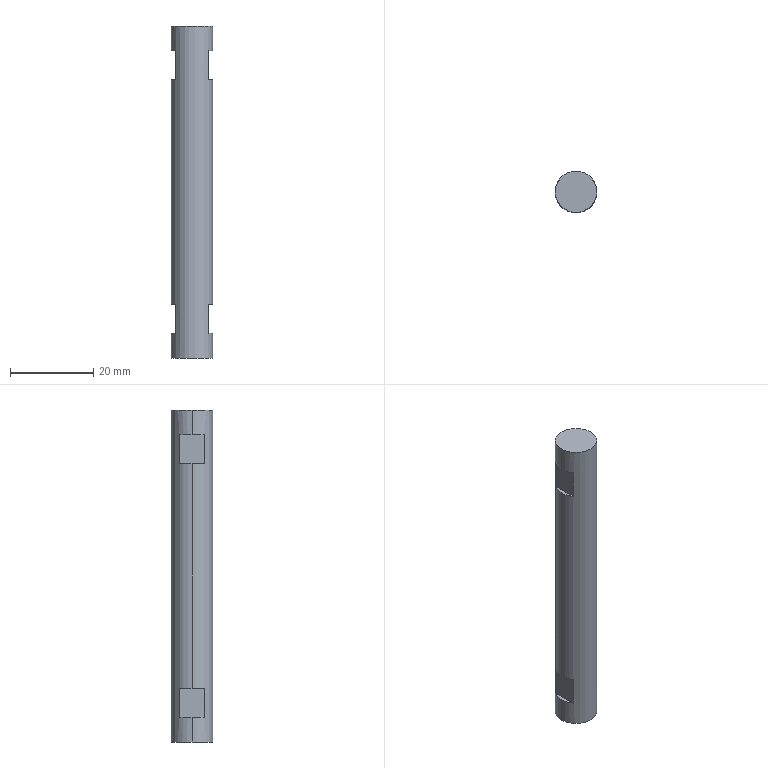Part | STEP file | GLSJ-10-19_default | 1 solid | 20 faces | box 10 x 10 x 80 mm | volume 5991 mm3 | plane 14 | cylinder 4 | cone 2 | commonest cylinder face diameters 4.2 x2 10 x2
STEP:
#1=CARTESIAN_POINT('',(0.,0.,0.));
#2=DIRECTION('',(0.,0.,1.));
#3=DIRECTION('',(1.,0.,0.));
#4=AXIS2_PLACEMENT_3D('',#1,#2,#3);
#5=CARTESIAN_POINT('',(-2.1,0.,12.4));
#6=VERTEX_POINT('',#5);
#7=CARTESIAN_POINT('',(-2.1,0.,0.));
#8=VERTEX_POINT('',#7);
#9=CARTESIAN_POINT('',(-2.1,0.,0.));
#10=DIRECTION('',(0.,0.,-1.));
#11=VECTOR('',#10,1.);
#12=LINE('',#9,#11);
#13=CARTESIAN_POINT('',(0.,0.,0.));
#14=DIRECTION('',(0.,0.,-1.));
#15=DIRECTION('',(-1.,0.,0.));
#16=AXIS2_PLACEMENT_3D('',#13,#14,#15);
#17=CYLINDRICAL_SURFACE('',#16,2.1);
#18=CARTESIAN_POINT('',(6.283,0.));
#19=DIRECTION('',(0.,1.));
#20=VECTOR('',#19,1.);
#21=LINE('',#18,#20);
#22=(GEOMETRIC_REPRESENTATION_CONTEXT(2)PARAMETRIC_REPRESENTATION_CONTEXT()REPRESENTATION_CONTEXT('',''));
#23=DEFINITIONAL_REPRESENTATION('',(#21),#22);
#24=PCURVE('',#17,#23);
#25=CARTESIAN_POINT('',(0.,0.,0.));
#26=DIRECTION('',(0.,0.,-1.));
#27=DIRECTION('',(-1.,0.,0.));
#28=AXIS2_PLACEMENT_3D('',#25,#26,#27);
#29=CYLINDRICAL_SURFACE('',#28,2.1);
#30=CARTESIAN_POINT('',(0.,0.));
#31=DIRECTION('',(0.,1.));
#32=VECTOR('',#31,1.);
#33=LINE('',#30,#32);
#34=(GEOMETRIC_REPRESENTATION_CONTEXT(2)PARAMETRIC_REPRESENTATION_CONTEXT()REPRESENTATION_CONTEXT('',''));
#35=DEFINITIONAL_REPRESENTATION('',(#33),#34);
#36=PCURVE('',#29,#35);
#37=SURFACE_CURVE('',#12,(#24,#36),.PCURVE_S1.);
#38=EDGE_CURVE('',#6,#8,#37,.T.);
#39=ORIENTED_EDGE('',*,*,#38,.T.);
#40=CARTESIAN_POINT('',(2.1,0.,0.));
#41=VERTEX_POINT('',#40);
#42=CARTESIAN_POINT('',(0.,0.,0.));
#43=DIRECTION('',(0.,0.,-1.));
#44=DIRECTION('',(-1.,0.,0.));
#45=AXIS2_PLACEMENT_3D('',#42,#43,#44);
#46=CIRCLE('',#45,2.1);
#47=CARTESIAN_POINT('',(0.,0.));
#48=DIRECTION('',(1.,0.));
#49=VECTOR('',#48,1.);
#50=LINE('',#47,#49);
#51=(GEOMETRIC_REPRESENTATION_CONTEXT(2)PARAMETRIC_REPRESENTATION_CONTEXT()REPRESENTATION_CONTEXT('',''));
#52=DEFINITIONAL_REPRESENTATION('',(#50),#51);
#53=PCURVE('',#17,#52);
#54=CARTESIAN_POINT('',(0.,0.,0.));
#55=DIRECTION('',(0.,0.,1.));
#56=DIRECTION('',(1.,0.,0.));
#57=AXIS2_PLACEMENT_3D('',#54,#55,#56);
#58=PLANE('',#57);
#59=CARTESIAN_POINT('',(-2.1,0.));
#60=CARTESIAN_POINT('',(-2.1,3.637));
#61=CARTESIAN_POINT('',(1.05,1.819));
#62=CARTESIAN_POINT('',(4.2,0.));
#63=CARTESIAN_POINT('',(1.05,-1.819));
#64=CARTESIAN_POINT('',(-2.1,-3.637));
#65=CARTESIAN_POINT('',(-2.1,0.));
#66=(BOUNDED_CURVE()B_SPLINE_CURVE(2,(#59,#60,#61,#62,#63,#64,#65),.UNSPECIFIED.,.T.,.F.)B_SPLINE_CURVE_WITH_KNOTS((1,2,2,2,2,1),(-2.094,0.,2.094,4.189,6.283,8.378),.UNSPECIFIED.)CURVE()GEOMETRIC_REPRESENTATION_ITEM()RATIONAL_B_SPLINE_CURVE((1.,0.5,1.,0.5,1.,0.5,1.))REPRESENTATION_ITEM(''));
#67=(GEOMETRIC_REPRESENTATION_CONTEXT(2)PARAMETRIC_REPRESENTATION_CONTEXT()REPRESENTATION_CONTEXT('',''));
#68=DEFINITIONAL_REPRESENTATION('',(#66),#67);
#69=PCURVE('',#58,#68);
#70=SURFACE_CURVE('',#46,(#53,#69),.PCURVE_S1.);
#71=EDGE_CURVE('',#41,#8,#70,.T.);
#72=ORIENTED_EDGE('',*,*,#71,.F.);
#73=CARTESIAN_POINT('',(2.1,0.,12.4));
#74=VERTEX_POINT('',#73);
#75=CARTESIAN_POINT('',(2.1,0.,0.));
#76=DIRECTION('',(0.,0.,-1.));
#77=VECTOR('',#76,1.);
#78=LINE('',#75,#77);
#79=CARTESIAN_POINT('',(3.142,0.));
#80=DIRECTION('',(0.,1.));
#81=VECTOR('',#80,1.);
#82=LINE('',#79,#81);
#83=(GEOMETRIC_REPRESENTATION_CONTEXT(2)PARAMETRIC_REPRESENTATION_CONTEXT()REPRESENTATION_CONTEXT('',''));
#84=DEFINITIONAL_REPRESENTATION('',(#82),#83);
#85=PCURVE('',#17,#84);
#86=CARTESIAN_POINT('',(3.142,0.));
#87=DIRECTION('',(0.,1.));
#88=VECTOR('',#87,1.);
#89=LINE('',#86,#88);
#90=(GEOMETRIC_REPRESENTATION_CONTEXT(2)PARAMETRIC_REPRESENTATION_CONTEXT()REPRESENTATION_CONTEXT('',''));
#91=DEFINITIONAL_REPRESENTATION('',(#89),#90);
#92=PCURVE('',#29,#91);
#93=SURFACE_CURVE('',#78,(#85,#92),.PCURVE_S1.);
#94=EDGE_CURVE('',#74,#41,#93,.T.);
#95=ORIENTED_EDGE('',*,*,#94,.F.);
#96=CARTESIAN_POINT('',(0.,0.,12.4));
#97=DIRECTION('',(0.,0.,-1.));
#98=DIRECTION('',(-1.,0.,0.));
#99=AXIS2_PLACEMENT_3D('',#96,#97,#98);
#100=CIRCLE('',#99,2.1);
#101=CARTESIAN_POINT('',(0.,-12.4));
#102=DIRECTION('',(1.,0.));
#103=VECTOR('',#102,1.);
#104=LINE('',#101,#103);
#105=(GEOMETRIC_REPRESENTATION_CONTEXT(2)PARAMETRIC_REPRESENTATION_CONTEXT()REPRESENTATION_CONTEXT('',''));
#106=DEFINITIONAL_REPRESENTATION('',(#104),#105);
#107=PCURVE('',#17,#106);
#108=CARTESIAN_POINT('',(0.,0.,12.4));
#109=DIRECTION('',(0.,0.,-1.));
#110=DIRECTION('',(-1.,0.,0.));
#111=AXIS2_PLACEMENT_3D('',#108,#109,#110);
#112=CONICAL_SURFACE('',#111,2.1,1.03);
#113=CARTESIAN_POINT('',(0.,0.));
#114=DIRECTION('',(1.,0.));
#115=VECTOR('',#114,1.);
#116=LINE('',#113,#115);
#117=(GEOMETRIC_REPRESENTATION_CONTEXT(2)PARAMETRIC_REPRESENTATION_CONTEXT()REPRESENTATION_CONTEXT('',''));
#118=DEFINITIONAL_REPRESENTATION('',(#116),#117);
#119=PCURVE('',#112,#118);
#120=SURFACE_CURVE('',#100,(#107,#119),.PCURVE_S1.);
#121=EDGE_CURVE('',#74,#6,#120,.T.);
#122=ORIENTED_EDGE('',*,*,#121,.T.);
#123=EDGE_LOOP('',(#39,#72,#95,#122));
#124=FACE_BOUND('',#123,.F.);
#125=ADVANCED_FACE('',(#124),#17,.F.);
#126=ORIENTED_EDGE('',*,*,#121,.F.);
#127=CARTESIAN_POINT('',(0.,0.,13.662));
#128=VERTEX_POINT('',#127);
#129=CARTESIAN_POINT('',(2.1,0.,12.4));
#130=DIRECTION('',(0.8572,0.,-0.515));
#131=VECTOR('',#130,1.);
#132=LINE('',#129,#131);
#133=CARTESIAN_POINT('',(3.142,-1.262));
#134=CARTESIAN_POINT('',(3.142,-1.243));
#135=CARTESIAN_POINT('',(3.142,-1.204));
#136=CARTESIAN_POINT('',(3.142,-1.147));
#137=CARTESIAN_POINT('',(3.142,-1.09));
#138=CARTESIAN_POINT('',(3.142,-1.032));
#139=CARTESIAN_POINT('',(3.142,-0.975));
#140=CARTESIAN_POINT('',(3.142,-0.9177));
#141=CARTESIAN_POINT('',(3.142,-0.8603));
#142=CARTESIAN_POINT('',(3.142,-0.803));
#143=CARTESIAN_POINT('',(3.142,-0.7456));
#144=CARTESIAN_POINT('',(3.142,-0.6883));
#145=CARTESIAN_POINT('',(3.142,-0.6309));
#146=CARTESIAN_POINT('',(3.142,-0.5735));
#147=CARTESIAN_POINT('',(3.142,-0.5162));
#148=CARTESIAN_POINT('',(3.142,-0.4588));
#149=CARTESIAN_POINT('',(3.142,-0.4015));
#150=CARTESIAN_POINT('',(3.142,-0.3441));
#151=CARTESIAN_POINT('',(3.142,-0.2868));
#152=CARTESIAN_POINT('',(3.142,-0.2294));
#153=CARTESIAN_POINT('',(3.142,-0.1721));
#154=CARTESIAN_POINT('',(3.142,-0.1147));
#155=CARTESIAN_POINT('',(3.142,-0.05735));
#156=CARTESIAN_POINT('',(3.142,-0.01912));
#157=CARTESIAN_POINT('',(3.142,0.));
#158=B_SPLINE_CURVE_WITH_KNOTS('',3,(#133,#134,#135,#136,#137,#138,#139,#140,#141,#142,#143,#144,#145,#146,#147,#148,#149,#150,#151,#152,#153,#154,#155,#156,#157),.UNSPECIFIED.,.F.,.F.,(4,1,1,1,1,1,1,1,1,1,1,1,1,1,1,1,1,1,1,1,1,1,4),(-2.45,-2.339,-2.227,-2.116,-2.004,-1.893,-1.782,-1.67,-1.559,-1.448,-1.336,-1.225,-1.114,-1.002,-0.8909,-0.7795,-0.6682,-0.5568,-0.4454,-0.3341,-0.2227,-0.1114,0.),.QUASI_UNIFORM_KNOTS.);
#159=(GEOMETRIC_REPRESENTATION_CONTEXT(2)PARAMETRIC_REPRESENTATION_CONTEXT()REPRESENTATION_CONTEXT('',''));
#160=DEFINITIONAL_REPRESENTATION('',(#158),#159);
#161=PCURVE('',#112,#160);
#162=CARTESIAN_POINT('',(0.,0.,12.4));
#163=DIRECTION('',(0.,0.,-1.));
#164=DIRECTION('',(-1.,0.,0.));
#165=AXIS2_PLACEMENT_3D('',#162,#163,#164);
#166=CONICAL_SURFACE('',#165,2.1,1.03);
#167=CARTESIAN_POINT('',(3.142,-1.262));
#168=CARTESIAN_POINT('',(3.142,-1.243));
#169=CARTESIAN_POINT('',(3.142,-1.204));
#170=CARTESIAN_POINT('',(3.142,-1.147));
#171=CARTESIAN_POINT('',(3.142,-1.09));
#172=CARTESIAN_POINT('',(3.142,-1.032));
#173=CARTESIAN_POINT('',(3.142,-0.975));
#174=CARTESIAN_POINT('',(3.142,-0.9177));
#175=CARTESIAN_POINT('',(3.142,-0.8603));
#176=CARTESIAN_POINT('',(3.142,-0.803));
#177=CARTESIAN_POINT('',(3.142,-0.7456));
#178=CARTESIAN_POINT('',(3.142,-0.6883));
#179=CARTESIAN_POINT('',(3.142,-0.6309));
#180=CARTESIAN_POINT('',(3.142,-0.5735));
#181=CARTESIAN_POINT('',(3.142,-0.5162));
#182=CARTESIAN_POINT('',(3.142,-0.4588));
#183=CARTESIAN_POINT('',(3.142,-0.4015));
#184=CARTESIAN_POINT('',(3.142,-0.3441));
#185=CARTESIAN_POINT('',(3.142,-0.2868));
#186=CARTESIAN_POINT('',(3.142,-0.2294));
#187=CARTESIAN_POINT('',(3.142,-0.1721));
#188=CARTESIAN_POINT('',(3.142,-0.1147));
#189=CARTESIAN_POINT('',(3.142,-0.05735));
#190=CARTESIAN_POINT('',(3.142,-0.01912));
#191=CARTESIAN_POINT('',(3.142,0.));
#192=B_SPLINE_CURVE_WITH_KNOTS('',3,(#167,#168,#169,#170,#171,#172,#173,#174,#175,#176,#177,#178,#179,#180,#181,#182,#183,#184,#185,#186,#187,#188,#189,#190,#191),.UNSPECIFIED.,.F.,.F.,(4,1,1,1,1,1,1,1,1,1,1,1,1,1,1,1,1,1,1,1,1,1,4),(-2.45,-2.339,-2.227,-2.116,-2.004,-1.893,-1.782,-1.67,-1.559,-1.448,-1.336,-1.225,-1.114,-1.002,-0.8909,-0.7795,-0.6682,-0.5568,-0.4454,-0.3341,-0.2227,-0.1114,0.),.QUASI_UNIFORM_KNOTS.);
#193=(GEOMETRIC_REPRESENTATION_CONTEXT(2)PARAMETRIC_REPRESENTATION_CONTEXT()REPRESENTATION_CONTEXT('',''));
#194=DEFINITIONAL_REPRESENTATION('',(#192),#193);
#195=PCURVE('',#166,#194);
#196=SURFACE_CURVE('',#132,(#161,#195),.PCURVE_S1.);
#197=EDGE_CURVE('',#128,#74,#196,.T.);
#198=ORIENTED_EDGE('',*,*,#197,.F.);
#199=CARTESIAN_POINT('',(-2.1,0.,12.4));
#200=DIRECTION('',(-0.8572,0.,-0.515));
#201=VECTOR('',#200,1.);
#202=LINE('',#199,#201);
#203=CARTESIAN_POINT('',(6.283,0.));
#204=DIRECTION('',(0.,1.));
#205=VECTOR('',#204,1.);
#206=LINE('',#203,#205);
#207=(GEOMETRIC_REPRESENTATION_CONTEXT(2)PARAMETRIC_REPRESENTATION_CONTEXT()REPRESENTATION_CONTEXT('',''));
#208=DEFINITIONAL_REPRESENTATION('',(#206),#207);
#209=PCURVE('',#112,#208);
#210=CARTESIAN_POINT('',(0.,0.));
#211=DIRECTION('',(0.,1.));
#212=VECTOR('',#211,1.);
#213=LINE('',#210,#212);
#214=(GEOMETRIC_REPRESENTATION_CONTEXT(2)PARAMETRIC_REPRESENTATION_CONTEXT()REPRESENTATION_CONTEXT('',''));
#215=DEFINITIONAL_REPRESENTATION('',(#213),#214);
#216=PCURVE('',#166,#215);
#217=SURFACE_CURVE('',#202,(#209,#216),.PCURVE_S1.);
#218=EDGE_CURVE('',#128,#6,#217,.T.);
#219=ORIENTED_EDGE('',*,*,#218,.T.);
#220=EDGE_LOOP('',(#126,#198,#219));
#221=FACE_BOUND('',#220,.F.);
#222=ADVANCED_FACE('',(#221),#112,.F.);
#223=CARTESIAN_POINT('',(5.,0.,80.));
#224=VERTEX_POINT('',#223);
#225=CARTESIAN_POINT('',(-5.,0.,80.));
#226=VERTEX_POINT('',#225);
#227=CARTESIAN_POINT('',(0.,0.,80.));
#228=DIRECTION('',(0.,0.,1.));
#229=DIRECTION('',(1.,0.,0.));
#230=AXIS2_PLACEMENT_3D('',#227,#228,#229);
#231=CIRCLE('',#230,5.);
#232=CARTESIAN_POINT('',(0.,0.,80.));
#233=DIRECTION('',(0.,0.,-1.));
#234=DIRECTION('',(-1.,0.,0.));
#235=AXIS2_PLACEMENT_3D('',#232,#233,#234);
#236=CYLINDRICAL_SURFACE('',#235,5.);
#237=CARTESIAN_POINT('',(3.142,0.));
#238=DIRECTION('',(-1.,0.));
#239=VECTOR('',#238,1.);
#240=LINE('',#237,#239);
#241=(GEOMETRIC_REPRESENTATION_CONTEXT(2)PARAMETRIC_REPRESENTATION_CONTEXT()REPRESENTATION_CONTEXT('',''));
#242=DEFINITIONAL_REPRESENTATION('',(#240),#241);
#243=PCURVE('',#236,#242);
#244=CARTESIAN_POINT('',(0.,0.,80.));
#245=DIRECTION('',(0.,0.,1.));
#246=DIRECTION('',(1.,0.,0.));
#247=AXIS2_PLACEMENT_3D('',#244,#245,#246);
#248=PLANE('',#247);
#249=CARTESIAN_POINT('',(0.,0.));
#250=DIRECTION('',(1.,0.));
#251=AXIS2_PLACEMENT_2D('',#249,#250);
#252=CIRCLE('',#251,5.);
#253=(GEOMETRIC_REPRESENTATION_CONTEXT(2)PARAMETRIC_REPRESENTATION_CONTEXT()REPRESENTATION_CONTEXT('',''));
#254=DEFINITIONAL_REPRESENTATION('',(#252),#253);
#255=PCURVE('',#248,#254);
#256=SURFACE_CURVE('',#231,(#243,#255),.PCURVE_S1.);
#257=EDGE_CURVE('',#224,#226,#256,.T.);
#258=ORIENTED_EDGE('',*,*,#257,.F.);
#259=CARTESIAN_POINT('',(5.,0.,74.));
#260=VERTEX_POINT('',#259);
#261=CARTESIAN_POINT('',(5.,0.,80.));
#262=DIRECTION('',(0.,0.,-1.));
#263=VECTOR('',#262,1.);
#264=LINE('',#261,#263);
#265=CARTESIAN_POINT('',(3.142,0.));
#266=DIRECTION('',(0.,1.));
#267=VECTOR('',#266,1.);
#268=LINE('',#265,#267);
#269=(GEOMETRIC_REPRESENTATION_CONTEXT(2)PARAMETRIC_REPRESENTATION_CONTEXT()REPRESENTATION_CONTEXT('',''));
#270=DEFINITIONAL_REPRESENTATION('',(#268),#269);
#271=PCURVE('',#236,#270);
#272=CARTESIAN_POINT('',(0.,0.,80.));
#273=DIRECTION('',(0.,0.,-1.));
#274=DIRECTION('',(-1.,0.,0.));
#275=AXIS2_PLACEMENT_3D('',#272,#273,#274);
#276=CYLINDRICAL_SURFACE('',#275,5.);
#277=CARTESIAN_POINT('',(3.142,0.));
#278=DIRECTION('',(0.,1.));
#279=VECTOR('',#278,1.);
#280=LINE('',#277,#279);
#281=(GEOMETRIC_REPRESENTATION_CONTEXT(2)PARAMETRIC_REPRESENTATION_CONTEXT()REPRESENTATION_CONTEXT('',''));
#282=DEFINITIONAL_REPRESENTATION('',(#280),#281);
#283=PCURVE('',#276,#282);
#284=SURFACE_CURVE('',#264,(#271,#283),.PCURVE_S1.);
#285=EDGE_CURVE('',#224,#260,#284,.T.);
#286=ORIENTED_EDGE('',*,*,#285,.T.);
#287=CARTESIAN_POINT('',(4.,3.,74.));
#288=VERTEX_POINT('',#287);
#289=CARTESIAN_POINT('',(0.,0.,74.));
#290=DIRECTION('',(0.,0.,1.));
#291=DIRECTION('',(1.,0.,0.));
#292=AXIS2_PLACEMENT_3D('',#289,#290,#291);
#293=CIRCLE('',#292,5.);
#294=CARTESIAN_POINT('',(3.142,6.));
#295=DIRECTION('',(-1.,0.));
#296=VECTOR('',#295,1.);
#297=LINE('',#294,#296);
#298=(GEOMETRIC_REPRESENTATION_CONTEXT(2)PARAMETRIC_REPRESENTATION_CONTEXT()REPRESENTATION_CONTEXT('',''));
#299=DEFINITIONAL_REPRESENTATION('',(#297),#298);
#300=PCURVE('',#236,#299);
#301=CARTESIAN_POINT('',(7.,-15.,74.));
#302=DIRECTION('',(0.,0.,1.));
#303=DIRECTION('',(1.,0.,0.));
#304=AXIS2_PLACEMENT_3D('',#301,#302,#303);
#305=PLANE('',#304);
#306=CARTESIAN_POINT('',(-7.,15.));
#307=DIRECTION('',(1.,0.));
#308=AXIS2_PLACEMENT_2D('',#306,#307);
#309=CIRCLE('',#308,5.);
#310=(GEOMETRIC_REPRESENTATION_CONTEXT(2)PARAMETRIC_REPRESENTATION_CONTEXT()REPRESENTATION_CONTEXT('',''));
#311=DEFINITIONAL_REPRESENTATION('',(#309),#310);
#312=PCURVE('',#305,#311);
#313=SURFACE_CURVE('',#293,(#300,#312),.PCURVE_S1.);
#314=EDGE_CURVE('',#260,#288,#313,.T.);
#315=ORIENTED_EDGE('',*,*,#314,.T.);
#316=CARTESIAN_POINT('',(4.,3.,67.));
#317=VERTEX_POINT('',#316);
#318=CARTESIAN_POINT('',(4.,3.,80.));
#319=DIRECTION('',(0.,0.,-1.));
#320=VECTOR('',#319,1.);
#321=LINE('',#318,#320);
#322=CARTESIAN_POINT('',(2.498,0.));
#323=DIRECTION('',(0.,1.));
#324=VECTOR('',#323,1.);
#325=LINE('',#322,#324);
#326=(GEOMETRIC_REPRESENTATION_CONTEXT(2)PARAMETRIC_REPRESENTATION_CONTEXT()REPRESENTATION_CONTEXT('',''));
#327=DEFINITIONAL_REPRESENTATION('',(#325),#326);
#328=PCURVE('',#236,#327);
#329=CARTESIAN_POINT('',(4.,-15.,74.));
#330=DIRECTION('',(-1.,0.,0.));
#331=DIRECTION('',(0.,0.,1.));
#332=AXIS2_PLACEMENT_3D('',#329,#330,#331);
#333=PLANE('',#332);
#334=CARTESIAN_POINT('',(6.,18.));
#335=DIRECTION('',(-1.,0.));
#336=VECTOR('',#335,1.);
#337=LINE('',#334,#336);
#338=(GEOMETRIC_REPRESENTATION_CONTEXT(2)PARAMETRIC_REPRESENTATION_CONTEXT()REPRESENTATION_CONTEXT('',''));
#339=DEFINITIONAL_REPRESENTATION('',(#337),#338);
#340=PCURVE('',#333,#339);
#341=SURFACE_CURVE('',#321,(#328,#340),.PCURVE_S1.);
#342=EDGE_CURVE('',#288,#317,#341,.T.);
#343=ORIENTED_EDGE('',*,*,#342,.T.);
#344=CARTESIAN_POINT('',(5.,0.,67.));
#345=VERTEX_POINT('',#344);
#346=CARTESIAN_POINT('',(0.,0.,67.));
#347=DIRECTION('',(0.,0.,-1.));
#348=DIRECTION('',(-1.,0.,0.));
#349=AXIS2_PLACEMENT_3D('',#346,#347,#348);
#350=CIRCLE('',#349,5.);
#351=CARTESIAN_POINT('',(0.,13.));
#352=DIRECTION('',(1.,0.));
#353=VECTOR('',#352,1.);
#354=LINE('',#351,#353);
#355=(GEOMETRIC_REPRESENTATION_CONTEXT(2)PARAMETRIC_REPRESENTATION_CONTEXT()REPRESENTATION_CONTEXT('',''));
#356=DEFINITIONAL_REPRESENTATION('',(#354),#355);
#357=PCURVE('',#236,#356);
#358=CARTESIAN_POINT('',(7.,-15.,67.));
#359=DIRECTION('',(0.,0.,-1.));
#360=DIRECTION('',(-1.,0.,0.));
#361=AXIS2_PLACEMENT_3D('',#358,#359,#360);
#362=PLANE('',#361);
#363=CARTESIAN_POINT('',(7.,15.));
#364=DIRECTION('',(1.,0.));
#365=AXIS2_PLACEMENT_2D('',#363,#364);
#366=CIRCLE('',#365,5.);
#367=(GEOMETRIC_REPRESENTATION_CONTEXT(2)PARAMETRIC_REPRESENTATION_CONTEXT()REPRESENTATION_CONTEXT('',''));
#368=DEFINITIONAL_REPRESENTATION('',(#366),#367);
#369=PCURVE('',#362,#368);
#370=SURFACE_CURVE('',#350,(#357,#369),.PCURVE_S1.);
#371=EDGE_CURVE('',#317,#345,#370,.T.);
#372=ORIENTED_EDGE('',*,*,#371,.T.);
#373=CARTESIAN_POINT('',(5.,0.,13.));
#374=VERTEX_POINT('',#373);
#375=CARTESIAN_POINT('',(5.,0.,80.));
#376=DIRECTION('',(0.,0.,-1.));
#377=VECTOR('',#376,1.);
#378=LINE('',#375,#377);
#379=CARTESIAN_POINT('',(3.142,0.));
#380=DIRECTION('',(0.,1.));
#381=VECTOR('',#380,1.);
#382=LINE('',#379,#381);
#383=(GEOMETRIC_REPRESENTATION_CONTEXT(2)PARAMETRIC_REPRESENTATION_CONTEXT()REPRESENTATION_CONTEXT('',''));
#384=DEFINITIONAL_REPRESENTATION('',(#382),#383);
#385=PCURVE('',#236,#384);
#386=CARTESIAN_POINT('',(3.142,0.));
#387=DIRECTION('',(0.,1.));
#388=VECTOR('',#387,1.);
#389=LINE('',#386,#388);
#390=(GEOMETRIC_REPRESENTATION_CONTEXT(2)PARAMETRIC_REPRESENTATION_CONTEXT()REPRESENTATION_CONTEXT('',''));
#391=DEFINITIONAL_REPRESENTATION('',(#389),#390);
#392=PCURVE('',#276,#391);
#393=SURFACE_CURVE('',#378,(#385,#392),.PCURVE_S1.);
#394=EDGE_CURVE('',#345,#374,#393,.T.);
#395=ORIENTED_EDGE('',*,*,#394,.T.);
#396=CARTESIAN_POINT('',(4.,3.,13.));
#397=VERTEX_POINT('',#396);
#398=CARTESIAN_POINT('',(0.,0.,13.));
#399=DIRECTION('',(0.,0.,1.));
#400=DIRECTION('',(1.,0.,0.));
#401=AXIS2_PLACEMENT_3D('',#398,#399,#400);
#402=CIRCLE('',#401,5.);
#403=CARTESIAN_POINT('',(3.142,67.));
#404=DIRECTION('',(-1.,0.));
#405=VECTOR('',#404,1.);
#406=LINE('',#403,#405);
#407=(GEOMETRIC_REPRESENTATION_CONTEXT(2)PARAMETRIC_REPRESENTATION_CONTEXT()REPRESENTATION_CONTEXT('',''));
#408=DEFINITIONAL_REPRESENTATION('',(#406),#407);
#409=PCURVE('',#236,#408);
#410=CARTESIAN_POINT('',(7.,-15.,13.));
#411=DIRECTION('',(0.,0.,1.));
#412=DIRECTION('',(1.,0.,0.));
#413=AXIS2_PLACEMENT_3D('',#410,#411,#412);
#414=PLANE('',#413);
#415=CARTESIAN_POINT('',(-7.,15.));
#416=DIRECTION('',(1.,0.));
#417=AXIS2_PLACEMENT_2D('',#415,#416);
#418=CIRCLE('',#417,5.);
#419=(GEOMETRIC_REPRESENTATION_CONTEXT(2)PARAMETRIC_REPRESENTATION_CONTEXT()REPRESENTATION_CONTEXT('',''));
#420=DEFINITIONAL_REPRESENTATION('',(#418),#419);
#421=PCURVE('',#414,#420);
#422=SURFACE_CURVE('',#402,(#409,#421),.PCURVE_S1.);
#423=EDGE_CURVE('',#374,#397,#422,.T.);
#424=ORIENTED_EDGE('',*,*,#423,.T.);
#425=CARTESIAN_POINT('',(4.,3.,6.));
#426=VERTEX_POINT('',#425);
#427=CARTESIAN_POINT('',(4.,3.,80.));
#428=DIRECTION('',(0.,0.,-1.));
#429=VECTOR('',#428,1.);
#430=LINE('',#427,#429);
#431=CARTESIAN_POINT('',(2.498,0.));
#432=DIRECTION('',(0.,1.));
#433=VECTOR('',#432,1.);
#434=LINE('',#431,#433);
#435=(GEOMETRIC_REPRESENTATION_CONTEXT(2)PARAMETRIC_REPRESENTATION_CONTEXT()REPRESENTATION_CONTEXT('',''));
#436=DEFINITIONAL_REPRESENTATION('',(#434),#435);
#437=PCURVE('',#236,#436);
#438=CARTESIAN_POINT('',(4.,-15.,6.));
#439=DIRECTION('',(-1.,0.,0.));
#440=DIRECTION('',(0.,0.,1.));
#441=AXIS2_PLACEMENT_3D('',#438,#439,#440);
#442=PLANE('',#441);
#443=CARTESIAN_POINT('',(74.,18.));
#444=DIRECTION('',(-1.,0.));
#445=VECTOR('',#444,1.);
#446=LINE('',#443,#445);
#447=(GEOMETRIC_REPRESENTATION_CONTEXT(2)PARAMETRIC_REPRESENTATION_CONTEXT()REPRESENTATION_CONTEXT('',''));
#448=DEFINITIONAL_REPRESENTATION('',(#446),#447);
#449=PCURVE('',#442,#448);
#450=SURFACE_CURVE('',#430,(#437,#449),.PCURVE_S1.);
#451=EDGE_CURVE('',#397,#426,#450,.T.);
#452=ORIENTED_EDGE('',*,*,#451,.T.);
#453=CARTESIAN_POINT('',(5.,0.,6.));
#454=VERTEX_POINT('',#453);
#455=CARTESIAN_POINT('',(0.,0.,6.));
#456=DIRECTION('',(0.,0.,-1.));
#457=DIRECTION('',(-1.,0.,0.));
#458=AXIS2_PLACEMENT_3D('',#455,#456,#457);
#459=CIRCLE('',#458,5.);
#460=CARTESIAN_POINT('',(0.,74.));
#461=DIRECTION('',(1.,0.));
#462=VECTOR('',#461,1.);
#463=LINE('',#460,#462);
#464=(GEOMETRIC_REPRESENTATION_CONTEXT(2)PARAMETRIC_REPRESENTATION_CONTEXT()REPRESENTATION_CONTEXT('',''));
#465=DEFINITIONAL_REPRESENTATION('',(#463),#464);
#466=PCURVE('',#236,#465);
#467=CARTESIAN_POINT('',(7.,-15.,6.));
#468=DIRECTION('',(0.,0.,-1.));
#469=DIRECTION('',(-1.,0.,0.));
#470=AXIS2_PLACEMENT_3D('',#467,#468,#469);
#471=PLANE('',#470);
#472=CARTESIAN_POINT('',(7.,15.));
#473=DIRECTION('',(1.,0.));
#474=AXIS2_PLACEMENT_2D('',#472,#473);
#475=CIRCLE('',#474,5.);
#476=(GEOMETRIC_REPRESENTATION_CONTEXT(2)PARAMETRIC_REPRESENTATION_CONTEXT()REPRESENTATION_CONTEXT('',''));
#477=DEFINITIONAL_REPRESENTATION('',(#475),#476);
#478=PCURVE('',#471,#477);
#479=SURFACE_CURVE('',#459,(#466,#478),.PCURVE_S1.);
#480=EDGE_CURVE('',#426,#454,#479,.T.);
#481=ORIENTED_EDGE('',*,*,#480,.T.);
#482=CARTESIAN_POINT('',(5.,0.,0.));
#483=VERTEX_POINT('',#482);
#484=CARTESIAN_POINT('',(5.,0.,80.));
#485=DIRECTION('',(0.,0.,-1.));
#486=VECTOR('',#485,1.);
#487=LINE('',#484,#486);
#488=CARTESIAN_POINT('',(3.142,0.));
#489=DIRECTION('',(0.,1.));
#490=VECTOR('',#489,1.);
#491=LINE('',#488,#490);
#492=(GEOMETRIC_REPRESENTATION_CONTEXT(2)PARAMETRIC_REPRESENTATION_CONTEXT()REPRESENTATION_CONTEXT('',''));
#493=DEFINITIONAL_REPRESENTATION('',(#491),#492);
#494=PCURVE('',#236,#493);
#495=CARTESIAN_POINT('',(3.142,0.));
#496=DIRECTION('',(0.,1.));
#497=VECTOR('',#496,1.);
#498=LINE('',#495,#497);
#499=(GEOMETRIC_REPRESENTATION_CONTEXT(2)PARAMETRIC_REPRESENTATION_CONTEXT()REPRESENTATION_CONTEXT('',''));
#500=DEFINITIONAL_REPRESENTATION('',(#498),#499);
#501=PCURVE('',#276,#500);
#502=SURFACE_CURVE('',#487,(#494,#501),.PCURVE_S1.);
#503=EDGE_CURVE('',#454,#483,#502,.T.);
#504=ORIENTED_EDGE('',*,*,#503,.T.);
#505=CARTESIAN_POINT('',(-5.,0.,0.));
#506=VERTEX_POINT('',#505);
#507=CARTESIAN_POINT('',(0.,0.,0.));
#508=DIRECTION('',(0.,0.,1.));
#509=DIRECTION('',(1.,0.,0.));
#510=AXIS2_PLACEMENT_3D('',#507,#508,#509);
#511=CIRCLE('',#510,5.);
#512=CARTESIAN_POINT('',(3.142,80.));
#513=DIRECTION('',(-1.,0.));
#514=VECTOR('',#513,1.);
#515=LINE('',#512,#514);
#516=(GEOMETRIC_REPRESENTATION_CONTEXT(2)PARAMETRIC_REPRESENTATION_CONTEXT()REPRESENTATION_CONTEXT('',''));
#517=DEFINITIONAL_REPRESENTATION('',(#515),#516);
#518=PCURVE('',#236,#517);
#519=CARTESIAN_POINT('',(0.,0.));
#520=DIRECTION('',(1.,0.));
#521=AXIS2_PLACEMENT_2D('',#519,#520);
#522=CIRCLE('',#521,5.);
#523=(GEOMETRIC_REPRESENTATION_CONTEXT(2)PARAMETRIC_REPRESENTATION_CONTEXT()REPRESENTATION_CONTEXT('',''));
#524=DEFINITIONAL_REPRESENTATION('',(#522),#523);
#525=PCURVE('',#58,#524);
#526=SURFACE_CURVE('',#511,(#518,#525),.PCURVE_S1.);
#527=EDGE_CURVE('',#483,#506,#526,.T.);
#528=ORIENTED_EDGE('',*,*,#527,.T.);
#529=CARTESIAN_POINT('',(-5.,0.,6.));
#530=VERTEX_POINT('',#529);
#531=CARTESIAN_POINT('',(-5.,0.,80.));
#532=DIRECTION('',(0.,0.,-1.));
#533=VECTOR('',#532,1.);
#534=LINE('',#531,#533);
#535=CARTESIAN_POINT('',(0.,0.));
#536=DIRECTION('',(0.,1.));
#537=VECTOR('',#536,1.);
#538=LINE('',#535,#537);
#539=(GEOMETRIC_REPRESENTATION_CONTEXT(2)PARAMETRIC_REPRESENTATION_CONTEXT()REPRESENTATION_CONTEXT('',''));
#540=DEFINITIONAL_REPRESENTATION('',(#538),#539);
#541=PCURVE('',#236,#540);
#542=CARTESIAN_POINT('',(6.283,0.));
#543=DIRECTION('',(0.,1.));
#544=VECTOR('',#543,1.);
#545=LINE('',#542,#544);
#546=(GEOMETRIC_REPRESENTATION_CONTEXT(2)PARAMETRIC_REPRESENTATION_CONTEXT()REPRESENTATION_CONTEXT('',''));
#547=DEFINITIONAL_REPRESENTATION('',(#545),#546);
#548=PCURVE('',#276,#547);
#549=SURFACE_CURVE('',#534,(#541,#548),.PCURVE_S1.);
#550=EDGE_CURVE('',#530,#506,#549,.T.);
#551=ORIENTED_EDGE('',*,*,#550,.F.);
#552=CARTESIAN_POINT('',(-4.,3.,6.));
#553=VERTEX_POINT('',#552);
#554=CARTESIAN_POINT('',(0.,0.,6.));
#555=DIRECTION('',(0.,0.,-1.));
#556=DIRECTION('',(-1.,0.,0.));
#557=AXIS2_PLACEMENT_3D('',#554,#555,#556);
#558=CIRCLE('',#557,5.);
#559=CARTESIAN_POINT('',(0.,74.));
#560=DIRECTION('',(1.,0.));
#561=VECTOR('',#560,1.);
#562=LINE('',#559,#561);
#563=(GEOMETRIC_REPRESENTATION_CONTEXT(2)PARAMETRIC_REPRESENTATION_CONTEXT()REPRESENTATION_CONTEXT('',''));
#564=DEFINITIONAL_REPRESENTATION('',(#562),#563);
#565=PCURVE('',#236,#564);
#566=CARTESIAN_POINT('',(-7.,-15.,6.));
#567=DIRECTION('',(0.,0.,-1.));
#568=DIRECTION('',(-1.,0.,0.));
#569=AXIS2_PLACEMENT_3D('',#566,#567,#568);
#570=PLANE('',#569);
#571=CARTESIAN_POINT('',(-7.,15.));
#572=DIRECTION('',(1.,0.));
#573=AXIS2_PLACEMENT_2D('',#571,#572);
#574=CIRCLE('',#573,5.);
#575=(GEOMETRIC_REPRESENTATION_CONTEXT(2)PARAMETRIC_REPRESENTATION_CONTEXT()REPRESENTATION_CONTEXT('',''));
#576=DEFINITIONAL_REPRESENTATION('',(#574),#575);
#577=PCURVE('',#570,#576);
#578=SURFACE_CURVE('',#558,(#565,#577),.PCURVE_S1.);
#579=EDGE_CURVE('',#530,#553,#578,.T.);
#580=ORIENTED_EDGE('',*,*,#579,.T.);
#581=CARTESIAN_POINT('',(-4.,3.,13.));
#582=VERTEX_POINT('',#581);
#583=CARTESIAN_POINT('',(-4.,3.,80.));
#584=DIRECTION('',(0.,0.,1.));
#585=VECTOR('',#584,1.);
#586=LINE('',#583,#585);
#587=CARTESIAN_POINT('',(0.6435,0.));
#588=DIRECTION('',(0.,-1.));
#589=VECTOR('',#588,1.);
#590=LINE('',#587,#589);
#591=(GEOMETRIC_REPRESENTATION_CONTEXT(2)PARAMETRIC_REPRESENTATION_CONTEXT()REPRESENTATION_CONTEXT('',''));
#592=DEFINITIONAL_REPRESENTATION('',(#590),#591);
#593=PCURVE('',#236,#592);
#594=CARTESIAN_POINT('',(-4.,-15.,6.));
#595=DIRECTION('',(1.,0.,0.));
#596=DIRECTION('',(0.,0.,-1.));
#597=AXIS2_PLACEMENT_3D('',#594,#595,#596);
#598=PLANE('',#597);
#599=CARTESIAN_POINT('',(-74.,18.));
#600=DIRECTION('',(-1.,0.));
#601=VECTOR('',#600,1.);
#602=LINE('',#599,#601);
#603=(GEOMETRIC_REPRESENTATION_CONTEXT(2)PARAMETRIC_REPRESENTATION_CONTEXT()REPRESENTATION_CONTEXT('',''));
#604=DEFINITIONAL_REPRESENTATION('',(#602),#603);
#605=PCURVE('',#598,#604);
#606=SURFACE_CURVE('',#586,(#593,#605),.PCURVE_S1.);
#607=EDGE_CURVE('',#553,#582,#606,.T.);
#608=ORIENTED_EDGE('',*,*,#607,.T.);
#609=CARTESIAN_POINT('',(-5.,0.,13.));
#610=VERTEX_POINT('',#609);
#611=CARTESIAN_POINT('',(0.,0.,13.));
#612=DIRECTION('',(0.,0.,1.));
#613=DIRECTION('',(1.,0.,0.));
#614=AXIS2_PLACEMENT_3D('',#611,#612,#613);
#615=CIRCLE('',#614,5.);
#616=CARTESIAN_POINT('',(3.142,67.));
#617=DIRECTION('',(-1.,0.));
#618=VECTOR('',#617,1.);
#619=LINE('',#616,#618);
#620=(GEOMETRIC_REPRESENTATION_CONTEXT(2)PARAMETRIC_REPRESENTATION_CONTEXT()REPRESENTATION_CONTEXT('',''));
#621=DEFINITIONAL_REPRESENTATION('',(#619),#620);
#622=PCURVE('',#236,#621);
#623=CARTESIAN_POINT('',(-7.,-15.,13.));
#624=DIRECTION('',(0.,0.,1.));
#625=DIRECTION('',(1.,0.,0.));
#626=AXIS2_PLACEMENT_3D('',#623,#624,#625);
#627=PLANE('',#626);
#628=CARTESIAN_POINT('',(7.,15.));
#629=DIRECTION('',(1.,0.));
#630=AXIS2_PLACEMENT_2D('',#628,#629);
#631=CIRCLE('',#630,5.);
#632=(GEOMETRIC_REPRESENTATION_CONTEXT(2)PARAMETRIC_REPRESENTATION_CONTEXT()REPRESENTATION_CONTEXT('',''));
#633=DEFINITIONAL_REPRESENTATION('',(#631),#632);
#634=PCURVE('',#627,#633);
#635=SURFACE_CURVE('',#615,(#622,#634),.PCURVE_S1.);
#636=EDGE_CURVE('',#582,#610,#635,.T.);
#637=ORIENTED_EDGE('',*,*,#636,.T.);
#638=CARTESIAN_POINT('',(-5.,0.,67.));
#639=VERTEX_POINT('',#638);
#640=CARTESIAN_POINT('',(-5.,0.,80.));
#641=DIRECTION('',(0.,0.,-1.));
#642=VECTOR('',#641,1.);
#643=LINE('',#640,#642);
#644=CARTESIAN_POINT('',(0.,0.));
#645=DIRECTION('',(0.,1.));
#646=VECTOR('',#645,1.);
#647=LINE('',#644,#646);
#648=(GEOMETRIC_REPRESENTATION_CONTEXT(2)PARAMETRIC_REPRESENTATION_CONTEXT()REPRESENTATION_CONTEXT('',''));
#649=DEFINITIONAL_REPRESENTATION('',(#647),#648);
#650=PCURVE('',#236,#649);
#651=CARTESIAN_POINT('',(6.283,0.));
#652=DIRECTION('',(0.,1.));
#653=VECTOR('',#652,1.);
#654=LINE('',#651,#653);
#655=(GEOMETRIC_REPRESENTATION_CONTEXT(2)PARAMETRIC_REPRESENTATION_CONTEXT()REPRESENTATION_CONTEXT('',''));
#656=DEFINITIONAL_REPRESENTATION('',(#654),#655);
#657=PCURVE('',#276,#656);
#658=SURFACE_CURVE('',#643,(#650,#657),.PCURVE_S1.);
#659=EDGE_CURVE('',#639,#610,#658,.T.);
#660=ORIENTED_EDGE('',*,*,#659,.F.);
#661=CARTESIAN_POINT('',(-4.,3.,67.));
#662=VERTEX_POINT('',#661);
#663=CARTESIAN_POINT('',(0.,0.,67.));
#664=DIRECTION('',(0.,0.,-1.));
#665=DIRECTION('',(-1.,0.,0.));
#666=AXIS2_PLACEMENT_3D('',#663,#664,#665);
#667=CIRCLE('',#666,5.);
#668=CARTESIAN_POINT('',(0.,13.));
#669=DIRECTION('',(1.,0.));
#670=VECTOR('',#669,1.);
#671=LINE('',#668,#670);
#672=(GEOMETRIC_REPRESENTATION_CONTEXT(2)PARAMETRIC_REPRESENTATION_CONTEXT()REPRESENTATION_CONTEXT('',''));
#673=DEFINITIONAL_REPRESENTATION('',(#671),#672);
#674=PCURVE('',#236,#673);
#675=CARTESIAN_POINT('',(-7.,-15.,67.));
#676=DIRECTION('',(0.,0.,-1.));
#677=DIRECTION('',(-1.,0.,0.));
#678=AXIS2_PLACEMENT_3D('',#675,#676,#677);
#679=PLANE('',#678);
#680=CARTESIAN_POINT('',(-7.,15.));
#681=DIRECTION('',(1.,0.));
#682=AXIS2_PLACEMENT_2D('',#680,#681);
#683=CIRCLE('',#682,5.);
#684=(GEOMETRIC_REPRESENTATION_CONTEXT(2)PARAMETRIC_REPRESENTATION_CONTEXT()REPRESENTATION_CONTEXT('',''));
#685=DEFINITIONAL_REPRESENTATION('',(#683),#684);
#686=PCURVE('',#679,#685);
#687=SURFACE_CURVE('',#667,(#674,#686),.PCURVE_S1.);
#688=EDGE_CURVE('',#639,#662,#687,.T.);
#689=ORIENTED_EDGE('',*,*,#688,.T.);
#690=CARTESIAN_POINT('',(-4.,3.,74.));
#691=VERTEX_POINT('',#690);
#692=CARTESIAN_POINT('',(-4.,3.,80.));
#693=DIRECTION('',(0.,0.,1.));
#694=VECTOR('',#693,1.);
#695=LINE('',#692,#694);
#696=CARTESIAN_POINT('',(0.6435,0.));
#697=DIRECTION('',(0.,-1.));
#698=VECTOR('',#697,1.);
#699=LINE('',#696,#698);
#700=(GEOMETRIC_REPRESENTATION_CONTEXT(2)PARAMETRIC_REPRESENTATION_CONTEXT()REPRESENTATION_CONTEXT('',''));
#701=DEFINITIONAL_REPRESENTATION('',(#699),#700);
#702=PCURVE('',#236,#701);
#703=CARTESIAN_POINT('',(-4.,-15.,74.));
#704=DIRECTION('',(1.,0.,0.));
#705=DIRECTION('',(0.,0.,-1.));
#706=AXIS2_PLACEMENT_3D('',#703,#704,#705);
#707=PLANE('',#706);
#708=CARTESIAN_POINT('',(-6.,18.));
#709=DIRECTION('',(-1.,0.));
#710=VECTOR('',#709,1.);
#711=LINE('',#708,#710);
#712=(GEOMETRIC_REPRESENTATION_CONTEXT(2)PARAMETRIC_REPRESENTATION_CONTEXT()REPRESENTATION_CONTEXT('',''));
#713=DEFINITIONAL_REPRESENTATION('',(#711),#712);
#714=PCURVE('',#707,#713);
#715=SURFACE_CURVE('',#695,(#702,#714),.PCURVE_S1.);
#716=EDGE_CURVE('',#662,#691,#715,.T.);
#717=ORIENTED_EDGE('',*,*,#716,.T.);
#718=CARTESIAN_POINT('',(-5.,0.,74.));
#719=VERTEX_POINT('',#718);
#720=CARTESIAN_POINT('',(0.,0.,74.));
#721=DIRECTION('',(0.,0.,1.));
#722=DIRECTION('',(1.,0.,0.));
#723=AXIS2_PLACEMENT_3D('',#720,#721,#722);
#724=CIRCLE('',#723,5.);
#725=CARTESIAN_POINT('',(3.142,6.));
#726=DIRECTION('',(-1.,0.));
#727=VECTOR('',#726,1.);
#728=LINE('',#725,#727);
#729=(GEOMETRIC_REPRESENTATION_CONTEXT(2)PARAMETRIC_REPRESENTATION_CONTEXT()REPRESENTATION_CONTEXT('',''));
#730=DEFINITIONAL_REPRESENTATION('',(#728),#729);
#731=PCURVE('',#236,#730);
#732=CARTESIAN_POINT('',(-7.,-15.,74.));
#733=DIRECTION('',(0.,0.,1.));
#734=DIRECTION('',(1.,0.,0.));
#735=AXIS2_PLACEMENT_3D('',#732,#733,#734);
#736=PLANE('',#735);
#737=CARTESIAN_POINT('',(7.,15.));
#738=DIRECTION('',(1.,0.));
#739=AXIS2_PLACEMENT_2D('',#737,#738);
#740=CIRCLE('',#739,5.);
#741=(GEOMETRIC_REPRESENTATION_CONTEXT(2)PARAMETRIC_REPRESENTATION_CONTEXT()REPRESENTATION_CONTEXT('',''));
#742=DEFINITIONAL_REPRESENTATION('',(#740),#741);
#743=PCURVE('',#736,#742);
#744=SURFACE_CURVE('',#724,(#731,#743),.PCURVE_S1.);
#745=EDGE_CURVE('',#691,#719,#744,.T.);
#746=ORIENTED_EDGE('',*,*,#745,.T.);
#747=CARTESIAN_POINT('',(-5.,0.,80.));
#748=DIRECTION('',(0.,0.,-1.));
#749=VECTOR('',#748,1.);
#750=LINE('',#747,#749);
#751=CARTESIAN_POINT('',(0.,0.));
#752=DIRECTION('',(0.,1.));
#753=VECTOR('',#752,1.);
#754=LINE('',#751,#753);
#755=(GEOMETRIC_REPRESENTATION_CONTEXT(2)PARAMETRIC_REPRESENTATION_CONTEXT()REPRESENTATION_CONTEXT('',''));
#756=DEFINITIONAL_REPRESENTATION('',(#754),#755);
#757=PCURVE('',#236,#756);
#758=CARTESIAN_POINT('',(6.283,0.));
#759=DIRECTION('',(0.,1.));
#760=VECTOR('',#759,1.);
#761=LINE('',#758,#760);
#762=(GEOMETRIC_REPRESENTATION_CONTEXT(2)PARAMETRIC_REPRESENTATION_CONTEXT()REPRESENTATION_CONTEXT('',''));
#763=DEFINITIONAL_REPRESENTATION('',(#761),#762);
#764=PCURVE('',#276,#763);
#765=SURFACE_CURVE('',#750,(#757,#764),.PCURVE_S1.);
#766=EDGE_CURVE('',#226,#719,#765,.T.);
#767=ORIENTED_EDGE('',*,*,#766,.F.);
#768=EDGE_LOOP('',(#258,#286,#315,#343,#372,#395,#424,#452,#481,#504,#528,#551,#580,#608,#637,#660,#689,#717,#746,#767));
#769=FACE_BOUND('',#768,.T.);
#770=ADVANCED_FACE('',(#769),#236,.T.);
#771=ORIENTED_EDGE('',*,*,#285,.F.);
#772=CARTESIAN_POINT('',(0.,0.,80.));
#773=DIRECTION('',(0.,0.,1.));
#774=DIRECTION('',(1.,0.,0.));
#775=AXIS2_PLACEMENT_3D('',#772,#773,#774);
#776=CIRCLE('',#775,5.);
#777=CARTESIAN_POINT('',(9.425,0.));
#778=DIRECTION('',(-1.,0.));
#779=VECTOR('',#778,1.);
#780=LINE('',#777,#779);
#781=(GEOMETRIC_REPRESENTATION_CONTEXT(2)PARAMETRIC_REPRESENTATION_CONTEXT()REPRESENTATION_CONTEXT('',''));
#782=DEFINITIONAL_REPRESENTATION('',(#780),#781);
#783=PCURVE('',#276,#782);
#784=CARTESIAN_POINT('',(0.,0.));
#785=DIRECTION('',(1.,0.));
#786=AXIS2_PLACEMENT_2D('',#784,#785);
#787=CIRCLE('',#786,5.);
#788=(GEOMETRIC_REPRESENTATION_CONTEXT(2)PARAMETRIC_REPRESENTATION_CONTEXT()REPRESENTATION_CONTEXT('',''));
#789=DEFINITIONAL_REPRESENTATION('',(#787),#788);
#790=PCURVE('',#248,#789);
#791=SURFACE_CURVE('',#776,(#783,#790),.PCURVE_S1.);
#792=EDGE_CURVE('',#226,#224,#791,.T.);
#793=ORIENTED_EDGE('',*,*,#792,.F.);
#794=ORIENTED_EDGE('',*,*,#766,.T.);
#795=CARTESIAN_POINT('',(-4.,-3.,74.));
#796=VERTEX_POINT('',#795);
#797=CARTESIAN_POINT('',(0.,0.,74.));
#798=DIRECTION('',(0.,0.,1.));
#799=DIRECTION('',(1.,0.,0.));
#800=AXIS2_PLACEMENT_3D('',#797,#798,#799);
#801=CIRCLE('',#800,5.);
#802=CARTESIAN_POINT('',(9.425,6.));
#803=DIRECTION('',(-1.,0.));
#804=VECTOR('',#803,1.);
#805=LINE('',#802,#804);
#806=(GEOMETRIC_REPRESENTATION_CONTEXT(2)PARAMETRIC_REPRESENTATION_CONTEXT()REPRESENTATION_CONTEXT('',''));
#807=DEFINITIONAL_REPRESENTATION('',(#805),#806);
#808=PCURVE('',#276,#807);
#809=CARTESIAN_POINT('',(7.,15.));
#810=DIRECTION('',(1.,0.));
#811=AXIS2_PLACEMENT_2D('',#809,#810);
#812=CIRCLE('',#811,5.);
#813=(GEOMETRIC_REPRESENTATION_CONTEXT(2)PARAMETRIC_REPRESENTATION_CONTEXT()REPRESENTATION_CONTEXT('',''));
#814=DEFINITIONAL_REPRESENTATION('',(#812),#813);
#815=PCURVE('',#736,#814);
#816=SURFACE_CURVE('',#801,(#808,#815),.PCURVE_S1.);
#817=EDGE_CURVE('',#719,#796,#816,.T.);
#818=ORIENTED_EDGE('',*,*,#817,.T.);
#819=CARTESIAN_POINT('',(-4.,-3.,67.));
#820=VERTEX_POINT('',#819);
#821=CARTESIAN_POINT('',(-4.,-3.,80.));
#822=DIRECTION('',(0.,0.,-1.));
#823=VECTOR('',#822,1.);
#824=LINE('',#821,#823);
#825=CARTESIAN_POINT('',(5.64,0.));
#826=DIRECTION('',(0.,1.));
#827=VECTOR('',#826,1.);
#828=LINE('',#825,#827);
#829=(GEOMETRIC_REPRESENTATION_CONTEXT(2)PARAMETRIC_REPRESENTATION_CONTEXT()REPRESENTATION_CONTEXT('',''));
#830=DEFINITIONAL_REPRESENTATION('',(#828),#829);
#831=PCURVE('',#276,#830);
#832=CARTESIAN_POINT('',(-6.,12.));
#833=DIRECTION('',(1.,0.));
#834=VECTOR('',#833,1.);
#835=LINE('',#832,#834);
#836=(GEOMETRIC_REPRESENTATION_CONTEXT(2)PARAMETRIC_REPRESENTATION_CONTEXT()REPRESENTATION_CONTEXT('',''));
#837=DEFINITIONAL_REPRESENTATION('',(#835),#836);
#838=PCURVE('',#707,#837);
#839=SURFACE_CURVE('',#824,(#831,#838),.PCURVE_S1.);
#840=EDGE_CURVE('',#796,#820,#839,.T.);
#841=ORIENTED_EDGE('',*,*,#840,.T.);
#842=CARTESIAN_POINT('',(0.,0.,67.));
#843=DIRECTION('',(0.,0.,-1.));
#844=DIRECTION('',(-1.,0.,0.));
#845=AXIS2_PLACEMENT_3D('',#842,#843,#844);
#846=CIRCLE('',#845,5.);
#847=CARTESIAN_POINT('',(0.,13.));
#848=DIRECTION('',(1.,0.));
#849=VECTOR('',#848,1.);
#850=LINE('',#847,#849);
#851=(GEOMETRIC_REPRESENTATION_CONTEXT(2)PARAMETRIC_REPRESENTATION_CONTEXT()REPRESENTATION_CONTEXT('',''));
#852=DEFINITIONAL_REPRESENTATION('',(#850),#851);
#853=PCURVE('',#276,#852);
#854=CARTESIAN_POINT('',(-7.,15.));
#855=DIRECTION('',(1.,0.));
#856=AXIS2_PLACEMENT_2D('',#854,#855);
#857=CIRCLE('',#856,5.);
#858=(GEOMETRIC_REPRESENTATION_CONTEXT(2)PARAMETRIC_REPRESENTATION_CONTEXT()REPRESENTATION_CONTEXT('',''));
#859=DEFINITIONAL_REPRESENTATION('',(#857),#858);
#860=PCURVE('',#679,#859);
#861=SURFACE_CURVE('',#846,(#853,#860),.PCURVE_S1.);
#862=EDGE_CURVE('',#820,#639,#861,.T.);
#863=ORIENTED_EDGE('',*,*,#862,.T.);
#864=ORIENTED_EDGE('',*,*,#659,.T.);
#865=CARTESIAN_POINT('',(-4.,-3.,13.));
#866=VERTEX_POINT('',#865);
#867=CARTESIAN_POINT('',(0.,0.,13.));
#868=DIRECTION('',(0.,0.,1.));
#869=DIRECTION('',(1.,0.,0.));
#870=AXIS2_PLACEMENT_3D('',#867,#868,#869);
#871=CIRCLE('',#870,5.);
#872=CARTESIAN_POINT('',(9.425,67.));
#873=DIRECTION('',(-1.,0.));
#874=VECTOR('',#873,1.);
#875=LINE('',#872,#874);
#876=(GEOMETRIC_REPRESENTATION_CONTEXT(2)PARAMETRIC_REPRESENTATION_CONTEXT()REPRESENTATION_CONTEXT('',''));
#877=DEFINITIONAL_REPRESENTATION('',(#875),#876);
#878=PCURVE('',#276,#877);
#879=CARTESIAN_POINT('',(7.,15.));
#880=DIRECTION('',(1.,0.));
#881=AXIS2_PLACEMENT_2D('',#879,#880);
#882=CIRCLE('',#881,5.);
#883=(GEOMETRIC_REPRESENTATION_CONTEXT(2)PARAMETRIC_REPRESENTATION_CONTEXT()REPRESENTATION_CONTEXT('',''));
#884=DEFINITIONAL_REPRESENTATION('',(#882),#883);
#885=PCURVE('',#627,#884);
#886=SURFACE_CURVE('',#871,(#878,#885),.PCURVE_S1.);
#887=EDGE_CURVE('',#610,#866,#886,.T.);
#888=ORIENTED_EDGE('',*,*,#887,.T.);
#889=CARTESIAN_POINT('',(-4.,-3.,6.));
#890=VERTEX_POINT('',#889);
#891=CARTESIAN_POINT('',(-4.,-3.,80.));
#892=DIRECTION('',(0.,0.,-1.));
#893=VECTOR('',#892,1.);
#894=LINE('',#891,#893);
#895=CARTESIAN_POINT('',(5.64,0.));
#896=DIRECTION('',(0.,1.));
#897=VECTOR('',#896,1.);
#898=LINE('',#895,#897);
#899=(GEOMETRIC_REPRESENTATION_CONTEXT(2)PARAMETRIC_REPRESENTATION_CONTEXT()REPRESENTATION_CONTEXT('',''));
#900=DEFINITIONAL_REPRESENTATION('',(#898),#899);
#901=PCURVE('',#276,#900);
#902=CARTESIAN_POINT('',(-74.,12.));
#903=DIRECTION('',(1.,0.));
#904=VECTOR('',#903,1.);
#905=LINE('',#902,#904);
#906=(GEOMETRIC_REPRESENTATION_CONTEXT(2)PARAMETRIC_REPRESENTATION_CONTEXT()REPRESENTATION_CONTEXT('',''));
#907=DEFINITIONAL_REPRESENTATION('',(#905),#906);
#908=PCURVE('',#598,#907);
#909=SURFACE_CURVE('',#894,(#901,#908),.PCURVE_S1.);
#910=EDGE_CURVE('',#866,#890,#909,.T.);
#911=ORIENTED_EDGE('',*,*,#910,.T.);
#912=CARTESIAN_POINT('',(0.,0.,6.));
#913=DIRECTION('',(0.,0.,-1.));
#914=DIRECTION('',(-1.,0.,0.));
#915=AXIS2_PLACEMENT_3D('',#912,#913,#914);
#916=CIRCLE('',#915,5.);
#917=CARTESIAN_POINT('',(0.,74.));
#918=DIRECTION('',(1.,0.));
#919=VECTOR('',#918,1.);
#920=LINE('',#917,#919);
#921=(GEOMETRIC_REPRESENTATION_CONTEXT(2)PARAMETRIC_REPRESENTATION_CONTEXT()REPRESENTATION_CONTEXT('',''));
#922=DEFINITIONAL_REPRESENTATION('',(#920),#921);
#923=PCURVE('',#276,#922);
#924=CARTESIAN_POINT('',(-7.,15.));
#925=DIRECTION('',(1.,0.));
#926=AXIS2_PLACEMENT_2D('',#924,#925);
#927=CIRCLE('',#926,5.);
#928=(GEOMETRIC_REPRESENTATION_CONTEXT(2)PARAMETRIC_REPRESENTATION_CONTEXT()REPRESENTATION_CONTEXT('',''));
#929=DEFINITIONAL_REPRESENTATION('',(#927),#928);
#930=PCURVE('',#570,#929);
#931=SURFACE_CURVE('',#916,(#923,#930),.PCURVE_S1.);
#932=EDGE_CURVE('',#890,#530,#931,.T.);
#933=ORIENTED_EDGE('',*,*,#932,.T.);
#934=ORIENTED_EDGE('',*,*,#550,.T.);
#935=CARTESIAN_POINT('',(0.,0.,0.));
#936=DIRECTION('',(0.,0.,1.));
#937=DIRECTION('',(1.,0.,0.));
#938=AXIS2_PLACEMENT_3D('',#935,#936,#937);
#939=CIRCLE('',#938,5.);
#940=CARTESIAN_POINT('',(9.425,80.));
#941=DIRECTION('',(-1.,0.));
#942=VECTOR('',#941,1.);
#943=LINE('',#940,#942);
#944=(GEOMETRIC_REPRESENTATION_CONTEXT(2)PARAMETRIC_REPRESENTATION_CONTEXT()REPRESENTATION_CONTEXT('',''));
#945=DEFINITIONAL_REPRESENTATION('',(#943),#944);
#946=PCURVE('',#276,#945);
#947=CARTESIAN_POINT('',(0.,0.));
#948=DIRECTION('',(1.,0.));
#949=AXIS2_PLACEMENT_2D('',#947,#948);
#950=CIRCLE('',#949,5.);
#951=(GEOMETRIC_REPRESENTATION_CONTEXT(2)PARAMETRIC_REPRESENTATION_CONTEXT()REPRESENTATION_CONTEXT('',''));
#952=DEFINITIONAL_REPRESENTATION('',(#950),#951);
#953=PCURVE('',#58,#952);
#954=SURFACE_CURVE('',#939,(#946,#953),.PCURVE_S1.);
#955=EDGE_CURVE('',#506,#483,#954,.T.);
#956=ORIENTED_EDGE('',*,*,#955,.T.);
#957=ORIENTED_EDGE('',*,*,#503,.F.);
#958=CARTESIAN_POINT('',(4.,-3.,6.));
#959=VERTEX_POINT('',#958);
#960=CARTESIAN_POINT('',(0.,0.,6.));
#961=DIRECTION('',(0.,0.,-1.));
#962=DIRECTION('',(-1.,0.,0.));
#963=AXIS2_PLACEMENT_3D('',#960,#961,#962);
#964=CIRCLE('',#963,5.);
#965=CARTESIAN_POINT('',(0.,74.));
#966=DIRECTION('',(1.,0.));
#967=VECTOR('',#966,1.);
#968=LINE('',#965,#967);
#969=(GEOMETRIC_REPRESENTATION_CONTEXT(2)PARAMETRIC_REPRESENTATION_CONTEXT()REPRESENTATION_CONTEXT('',''));
#970=DEFINITIONAL_REPRESENTATION('',(#968),#969);
#971=PCURVE('',#276,#970);
#972=CARTESIAN_POINT('',(7.,15.));
#973=DIRECTION('',(1.,0.));
#974=AXIS2_PLACEMENT_2D('',#972,#973);
#975=CIRCLE('',#974,5.);
#976=(GEOMETRIC_REPRESENTATION_CONTEXT(2)PARAMETRIC_REPRESENTATION_CONTEXT()REPRESENTATION_CONTEXT('',''));
#977=DEFINITIONAL_REPRESENTATION('',(#975),#976);
#978=PCURVE('',#471,#977);
#979=SURFACE_CURVE('',#964,(#971,#978),.PCURVE_S1.);
#980=EDGE_CURVE('',#454,#959,#979,.T.);
#981=ORIENTED_EDGE('',*,*,#980,.T.);
#982=CARTESIAN_POINT('',(4.,-3.,13.));
#983=VERTEX_POINT('',#982);
#984=CARTESIAN_POINT('',(4.,-3.,80.));
#985=DIRECTION('',(0.,0.,1.));
#986=VECTOR('',#985,1.);
#987=LINE('',#984,#986);
#988=CARTESIAN_POINT('',(3.785,0.));
#989=DIRECTION('',(0.,-1.));
#990=VECTOR('',#989,1.);
#991=LINE('',#988,#990);
#992=(GEOMETRIC_REPRESENTATION_CONTEXT(2)PARAMETRIC_REPRESENTATION_CONTEXT()REPRESENTATION_CONTEXT('',''));
#993=DEFINITIONAL_REPRESENTATION('',(#991),#992);
#994=PCURVE('',#276,#993);
#995=CARTESIAN_POINT('',(74.,12.));
#996=DIRECTION('',(1.,0.));
#997=VECTOR('',#996,1.);
#998=LINE('',#995,#997);
#999=(GEOMETRIC_REPRESENTATION_CONTEXT(2)PARAMETRIC_REPRESENTATION_CONTEXT()REPRESENTATION_CONTEXT('',''));
#1000=DEFINITIONAL_REPRESENTATION('',(#998),#999);
#1001=PCURVE('',#442,#1000);
#1002=SURFACE_CURVE('',#987,(#994,#1001),.PCURVE_S1.);
#1003=EDGE_CURVE('',#959,#983,#1002,.T.);
#1004=ORIENTED_EDGE('',*,*,#1003,.T.);
#1005=CARTESIAN_POINT('',(0.,0.,13.));
#1006=DIRECTION('',(0.,0.,1.));
#1007=DIRECTION('',(1.,0.,0.));
#1008=AXIS2_PLACEMENT_3D('',#1005,#1006,#1007);
#1009=CIRCLE('',#1008,5.);
#1010=CARTESIAN_POINT('',(9.425,67.));
#1011=DIRECTION('',(-1.,0.));
#1012=VECTOR('',#1011,1.);
#1013=LINE('',#1010,#1012);
#1014=(GEOMETRIC_REPRESENTATION_CONTEXT(2)PARAMETRIC_REPRESENTATION_CONTEXT()REPRESENTATION_CONTEXT('',''));
#1015=DEFINITIONAL_REPRESENTATION('',(#1013),#1014);
#1016=PCURVE('',#276,#1015);
#1017=CARTESIAN_POINT('',(-7.,15.));
#1018=DIRECTION('',(1.,0.));
#1019=AXIS2_PLACEMENT_2D('',#1017,#1018);
#1020=CIRCLE('',#1019,5.);
#1021=(GEOMETRIC_REPRESENTATION_CONTEXT(2)PARAMETRIC_REPRESENTATION_CONTEXT()REPRESENTATION_CONTEXT('',''));
#1022=DEFINITIONAL_REPRESENTATION('',(#1020),#1021);
#1023=PCURVE('',#414,#1022);
#1024=SURFACE_CURVE('',#1009,(#1016,#1023),.PCURVE_S1.);
#1025=EDGE_CURVE('',#983,#374,#1024,.T.);
#1026=ORIENTED_EDGE('',*,*,#1025,.T.);
#1027=ORIENTED_EDGE('',*,*,#394,.F.);
#1028=CARTESIAN_POINT('',(4.,-3.,67.));
#1029=VERTEX_POINT('',#1028);
#1030=CARTESIAN_POINT('',(0.,0.,67.));
#1031=DIRECTION('',(0.,0.,-1.));
#1032=DIRECTION('',(-1.,0.,0.));
#1033=AXIS2_PLACEMENT_3D('',#1030,#1031,#1032);
#1034=CIRCLE('',#1033,5.);
#1035=CARTESIAN_POINT('',(0.,13.));
#1036=DIRECTION('',(1.,0.));
#1037=VECTOR('',#1036,1.);
#1038=LINE('',#1035,#1037);
#1039=(GEOMETRIC_REPRESENTATION_CONTEXT(2)PARAMETRIC_REPRESENTATION_CONTEXT()REPRESENTATION_CONTEXT('',''));
#1040=DEFINITIONAL_REPRESENTATION('',(#1038),#1039);
#1041=PCURVE('',#276,#1040);
#1042=CARTESIAN_POINT('',(7.,15.));
#1043=DIRECTION('',(1.,0.));
#1044=AXIS2_PLACEMENT_2D('',#1042,#1043);
#1045=CIRCLE('',#1044,5.);
#1046=(GEOMETRIC_REPRESENTATION_CONTEXT(2)PARAMETRIC_REPRESENTATION_CONTEXT()REPRESENTATION_CONTEXT('',''));
#1047=DEFINITIONAL_REPRESENTATION('',(#1045),#1046);
#1048=PCURVE('',#362,#1047);
#1049=SURFACE_CURVE('',#1034,(#1041,#1048),.PCURVE_S1.);
#1050=EDGE_CURVE('',#345,#1029,#1049,.T.);
#1051=ORIENTED_EDGE('',*,*,#1050,.T.);
#1052=CARTESIAN_POINT('',(4.,-3.,74.));
#1053=VERTEX_POINT('',#1052);
#1054=CARTESIAN_POINT('',(4.,-3.,80.));
#1055=DIRECTION('',(0.,0.,1.));
#1056=VECTOR('',#1055,1.);
#1057=LINE('',#1054,#1056);
#1058=CARTESIAN_POINT('',(3.785,0.));
#1059=DIRECTION('',(0.,-1.));
#1060=VECTOR('',#1059,1.);
#1061=LINE('',#1058,#1060);
#1062=(GEOMETRIC_REPRESENTATION_CONTEXT(2)PARAMETRIC_REPRESENTATION_CONTEXT()REPRESENTATION_CONTEXT('',''));
#1063=DEFINITIONAL_REPRESENTATION('',(#1061),#1062);
#1064=PCURVE('',#276,#1063);
#1065=CARTESIAN_POINT('',(6.,12.));
#1066=DIRECTION('',(1.,0.));
#1067=VECTOR('',#1066,1.);
#1068=LINE('',#1065,#1067);
#1069=(GEOMETRIC_REPRESENTATION_CONTEXT(2)PARAMETRIC_REPRESENTATION_CONTEXT()REPRESENTATION_CONTEXT('',''));
#1070=DEFINITIONAL_REPRESENTATION('',(#1068),#1069);
#1071=PCURVE('',#333,#1070);
#1072=SURFACE_CURVE('',#1057,(#1064,#1071),.PCURVE_S1.);
#1073=EDGE_CURVE('',#1029,#1053,#1072,.T.);
#1074=ORIENTED_EDGE('',*,*,#1073,.T.);
#1075=CARTESIAN_POINT('',(0.,0.,74.));
#1076=DIRECTION('',(0.,0.,1.));
#1077=DIRECTION('',(1.,0.,0.));
#1078=AXIS2_PLACEMENT_3D('',#1075,#1076,#1077);
#1079=CIRCLE('',#1078,5.);
#1080=CARTESIAN_POINT('',(9.425,6.));
#1081=DIRECTION('',(-1.,0.));
#1082=VECTOR('',#1081,1.);
#1083=LINE('',#1080,#1082);
#1084=(GEOMETRIC_REPRESENTATION_CONTEXT(2)PARAMETRIC_REPRESENTATION_CONTEXT()REPRESENTATION_CONTEXT('',''));
#1085=DEFINITIONAL_REPRESENTATION('',(#1083),#1084);
#1086=PCURVE('',#276,#1085);
#1087=CARTESIAN_POINT('',(-7.,15.));
#1088=DIRECTION('',(1.,0.));
#1089=AXIS2_PLACEMENT_2D('',#1087,#1088);
#1090=CIRCLE('',#1089,5.);
#1091=(GEOMETRIC_REPRESENTATION_CONTEXT(2)PARAMETRIC_REPRESENTATION_CONTEXT()REPRESENTATION_CONTEXT('',''));
#1092=DEFINITIONAL_REPRESENTATION('',(#1090),#1091);
#1093=PCURVE('',#305,#1092);
#1094=SURFACE_CURVE('',#1079,(#1086,#1093),.PCURVE_S1.);
#1095=EDGE_CURVE('',#1053,#260,#1094,.T.);
#1096=ORIENTED_EDGE('',*,*,#1095,.T.);
#1097=EDGE_LOOP('',(#771,#793,#794,#818,#841,#863,#864,#888,#911,#933,#934,#956,#957,#981,#1004,#1026,#1027,#1051,#1074,#1096));
#1098=FACE_BOUND('',#1097,.T.);
#1099=ADVANCED_FACE('',(#1098),#276,.T.);
#1100=ORIENTED_EDGE('',*,*,#792,.T.);
#1101=ORIENTED_EDGE('',*,*,#257,.T.);
#1102=EDGE_LOOP('',(#1100,#1101));
#1103=FACE_BOUND('',#1102,.T.);
#1104=ADVANCED_FACE('',(#1103),#248,.T.);
#1105=CARTESIAN_POINT('',(0.,0.,0.));
#1106=DIRECTION('',(0.,0.,-1.));
#1107=DIRECTION('',(-1.,0.,0.));
#1108=AXIS2_PLACEMENT_3D('',#1105,#1106,#1107);
#1109=CIRCLE('',#1108,2.1);
#1110=CARTESIAN_POINT('',(-2.1,0.));
#1111=CARTESIAN_POINT('',(-2.1,3.637));
#1112=CARTESIAN_POINT('',(1.05,1.819));
#1113=CARTESIAN_POINT('',(4.2,0.));
#1114=CARTESIAN_POINT('',(1.05,-1.819));
#1115=CARTESIAN_POINT('',(-2.1,-3.637));
#1116=CARTESIAN_POINT('',(-2.1,0.));
#1117=(BOUNDED_CURVE()B_SPLINE_CURVE(2,(#1110,#1111,#1112,#1113,#1114,#1115,#1116),.UNSPECIFIED.,.T.,.F.)B_SPLINE_CURVE_WITH_KNOTS((1,2,2,2,2,1),(-2.094,0.,2.094,4.189,6.283,8.378),.UNSPECIFIED.)CURVE()GEOMETRIC_REPRESENTATION_ITEM()RATIONAL_B_SPLINE_CURVE((1.,0.5,1.,0.5,1.,0.5,1.))REPRESENTATION_ITEM(''));
#1118=(GEOMETRIC_REPRESENTATION_CONTEXT(2)PARAMETRIC_REPRESENTATION_CONTEXT()REPRESENTATION_CONTEXT('',''));
#1119=DEFINITIONAL_REPRESENTATION('',(#1117),#1118);
#1120=PCURVE('',#58,#1119);
#1121=CARTESIAN_POINT('',(0.,0.));
#1122=DIRECTION('',(1.,0.));
#1123=VECTOR('',#1122,1.);
#1124=LINE('',#1121,#1123);
#1125=(GEOMETRIC_REPRESENTATION_CONTEXT(2)PARAMETRIC_REPRESENTATION_CONTEXT()REPRESENTATION_CONTEXT('',''));
#1126=DEFINITIONAL_REPRESENTATION('',(#1124),#1125);
#1127=PCURVE('',#29,#1126);
#1128=SURFACE_CURVE('',#1109,(#1120,#1127),.PCURVE_S1.);
#1129=EDGE_CURVE('',#8,#41,#1128,.T.);
#1130=ORIENTED_EDGE('',*,*,#1129,.F.);
#1131=ORIENTED_EDGE('',*,*,#71,.F.);
#1132=EDGE_LOOP('',(#1130,#1131));
#1133=FACE_BOUND('',#1132,.T.);
#1134=ORIENTED_EDGE('',*,*,#955,.F.);
#1135=ORIENTED_EDGE('',*,*,#527,.F.);
#1136=EDGE_LOOP('',(#1134,#1135));
#1137=FACE_BOUND('',#1136,.T.);
#1138=ADVANCED_FACE('',(#1133,#1137),#58,.F.);
#1139=CARTESIAN_POINT('',(0.,0.,12.4));
#1140=DIRECTION('',(0.,0.,-1.));
#1141=DIRECTION('',(-1.,0.,0.));
#1142=AXIS2_PLACEMENT_3D('',#1139,#1140,#1141);
#1143=CIRCLE('',#1142,2.1);
#1144=CARTESIAN_POINT('',(0.,0.));
#1145=DIRECTION('',(1.,0.));
#1146=VECTOR('',#1145,1.);
#1147=LINE('',#1144,#1146);
#1148=(GEOMETRIC_REPRESENTATION_CONTEXT(2)PARAMETRIC_REPRESENTATION_CONTEXT()REPRESENTATION_CONTEXT('',''));
#1149=DEFINITIONAL_REPRESENTATION('',(#1147),#1148);
#1150=PCURVE('',#166,#1149);
#1151=CARTESIAN_POINT('',(0.,-12.4));
#1152=DIRECTION('',(1.,0.));
#1153=VECTOR('',#1152,1.);
#1154=LINE('',#1151,#1153);
#1155=(GEOMETRIC_REPRESENTATION_CONTEXT(2)PARAMETRIC_REPRESENTATION_CONTEXT()REPRESENTATION_CONTEXT('',''));
#1156=DEFINITIONAL_REPRESENTATION('',(#1154),#1155);
#1157=PCURVE('',#29,#1156);
#1158=SURFACE_CURVE('',#1143,(#1150,#1157),.PCURVE_S1.);
#1159=EDGE_CURVE('',#6,#74,#1158,.T.);
#1160=ORIENTED_EDGE('',*,*,#1159,.F.);
#1161=ORIENTED_EDGE('',*,*,#218,.F.);
#1162=ORIENTED_EDGE('',*,*,#197,.T.);
#1163=EDGE_LOOP('',(#1160,#1161,#1162));
#1164=FACE_BOUND('',#1163,.F.);
#1165=ADVANCED_FACE('',(#1164),#166,.F.);
#1166=ORIENTED_EDGE('',*,*,#1129,.F.);
#1167=ORIENTED_EDGE('',*,*,#38,.F.);
#1168=ORIENTED_EDGE('',*,*,#1159,.T.);
#1169=ORIENTED_EDGE('',*,*,#94,.T.);
#1170=EDGE_LOOP('',(#1166,#1167,#1168,#1169));
#1171=FACE_BOUND('',#1170,.F.);
#1172=ADVANCED_FACE('',(#1171),#29,.F.);
#1173=CARTESIAN_POINT('',(4.,-15.,13.));
#1174=DIRECTION('',(0.,1.,0.));
#1175=VECTOR('',#1174,1.);
#1176=LINE('',#1173,#1175);
#1177=CARTESIAN_POINT('',(-3.,0.));
#1178=DIRECTION('',(0.,1.));
#1179=VECTOR('',#1178,1.);
#1180=LINE('',#1177,#1179);
#1181=(GEOMETRIC_REPRESENTATION_CONTEXT(2)PARAMETRIC_REPRESENTATION_CONTEXT()REPRESENTATION_CONTEXT('',''));
#1182=DEFINITIONAL_REPRESENTATION('',(#1180),#1181);
#1183=PCURVE('',#414,#1182);
#1184=CARTESIAN_POINT('',(7.,0.));
#1185=DIRECTION('',(0.,1.));
#1186=VECTOR('',#1185,1.);
#1187=LINE('',#1184,#1186);
#1188=(GEOMETRIC_REPRESENTATION_CONTEXT(2)PARAMETRIC_REPRESENTATION_CONTEXT()REPRESENTATION_CONTEXT('',''));
#1189=DEFINITIONAL_REPRESENTATION('',(#1187),#1188);
#1190=PCURVE('',#442,#1189);
#1191=SURFACE_CURVE('',#1176,(#1183,#1190),.PCURVE_S1.);
#1192=EDGE_CURVE('',#983,#397,#1191,.T.);
#1193=ORIENTED_EDGE('',*,*,#1192,.T.);
#1194=ORIENTED_EDGE('',*,*,#423,.F.);
#1195=ORIENTED_EDGE('',*,*,#1025,.F.);
#1196=EDGE_LOOP('',(#1193,#1194,#1195));
#1197=FACE_BOUND('',#1196,.T.);
#1198=ADVANCED_FACE('',(#1197),#414,.F.);
#1199=ORIENTED_EDGE('',*,*,#1192,.F.);
#1200=ORIENTED_EDGE('',*,*,#1003,.F.);
#1201=CARTESIAN_POINT('',(4.,-15.,6.));
#1202=DIRECTION('',(0.,1.,0.));
#1203=VECTOR('',#1202,1.);
#1204=LINE('',#1201,#1203);
#1205=CARTESIAN_POINT('',(0.,0.));
#1206=DIRECTION('',(0.,1.));
#1207=VECTOR('',#1206,1.);
#1208=LINE('',#1205,#1207);
#1209=(GEOMETRIC_REPRESENTATION_CONTEXT(2)PARAMETRIC_REPRESENTATION_CONTEXT()REPRESENTATION_CONTEXT('',''));
#1210=DEFINITIONAL_REPRESENTATION('',(#1208),#1209);
#1211=PCURVE('',#442,#1210);
#1212=CARTESIAN_POINT('',(3.,0.));
#1213=DIRECTION('',(0.,1.));
#1214=VECTOR('',#1213,1.);
#1215=LINE('',#1212,#1214);
#1216=(GEOMETRIC_REPRESENTATION_CONTEXT(2)PARAMETRIC_REPRESENTATION_CONTEXT()REPRESENTATION_CONTEXT('',''));
#1217=DEFINITIONAL_REPRESENTATION('',(#1215),#1216);
#1218=PCURVE('',#471,#1217);
#1219=SURFACE_CURVE('',#1204,(#1211,#1218),.PCURVE_S1.);
#1220=EDGE_CURVE('',#959,#426,#1219,.T.);
#1221=ORIENTED_EDGE('',*,*,#1220,.T.);
#1222=ORIENTED_EDGE('',*,*,#451,.F.);
#1223=EDGE_LOOP('',(#1199,#1200,#1221,#1222));
#1224=FACE_BOUND('',#1223,.T.);
#1225=ADVANCED_FACE('',(#1224),#442,.F.);
#1226=ORIENTED_EDGE('',*,*,#1220,.F.);
#1227=ORIENTED_EDGE('',*,*,#980,.F.);
#1228=ORIENTED_EDGE('',*,*,#480,.F.);
#1229=EDGE_LOOP('',(#1226,#1227,#1228));
#1230=FACE_BOUND('',#1229,.T.);
#1231=ADVANCED_FACE('',(#1230),#471,.F.);
#1232=CARTESIAN_POINT('',(-4.,-15.,6.));
#1233=DIRECTION('',(0.,1.,0.));
#1234=VECTOR('',#1233,1.);
#1235=LINE('',#1232,#1234);
#1236=CARTESIAN_POINT('',(-3.,0.));
#1237=DIRECTION('',(0.,1.));
#1238=VECTOR('',#1237,1.);
#1239=LINE('',#1236,#1238);
#1240=(GEOMETRIC_REPRESENTATION_CONTEXT(2)PARAMETRIC_REPRESENTATION_CONTEXT()REPRESENTATION_CONTEXT('',''));
#1241=DEFINITIONAL_REPRESENTATION('',(#1239),#1240);
#1242=PCURVE('',#570,#1241);
#1243=CARTESIAN_POINT('',(0.,0.));
#1244=DIRECTION('',(0.,1.));
#1245=VECTOR('',#1244,1.);
#1246=LINE('',#1243,#1245);
#1247=(GEOMETRIC_REPRESENTATION_CONTEXT(2)PARAMETRIC_REPRESENTATION_CONTEXT()REPRESENTATION_CONTEXT('',''));
#1248=DEFINITIONAL_REPRESENTATION('',(#1246),#1247);
#1249=PCURVE('',#598,#1248);
#1250=SURFACE_CURVE('',#1235,(#1242,#1249),.PCURVE_S1.);
#1251=EDGE_CURVE('',#890,#553,#1250,.T.);
#1252=ORIENTED_EDGE('',*,*,#1251,.T.);
#1253=ORIENTED_EDGE('',*,*,#579,.F.);
#1254=ORIENTED_EDGE('',*,*,#932,.F.);
#1255=EDGE_LOOP('',(#1252,#1253,#1254));
#1256=FACE_BOUND('',#1255,.T.);
#1257=ADVANCED_FACE('',(#1256),#570,.F.);
#1258=CARTESIAN_POINT('',(-4.,-15.,13.));
#1259=DIRECTION('',(0.,1.,0.));
#1260=VECTOR('',#1259,1.);
#1261=LINE('',#1258,#1260);
#1262=CARTESIAN_POINT('',(-7.,0.));
#1263=DIRECTION('',(0.,1.));
#1264=VECTOR('',#1263,1.);
#1265=LINE('',#1262,#1264);
#1266=(GEOMETRIC_REPRESENTATION_CONTEXT(2)PARAMETRIC_REPRESENTATION_CONTEXT()REPRESENTATION_CONTEXT('',''));
#1267=DEFINITIONAL_REPRESENTATION('',(#1265),#1266);
#1268=PCURVE('',#598,#1267);
#1269=CARTESIAN_POINT('',(3.,0.));
#1270=DIRECTION('',(0.,1.));
#1271=VECTOR('',#1270,1.);
#1272=LINE('',#1269,#1271);
#1273=(GEOMETRIC_REPRESENTATION_CONTEXT(2)PARAMETRIC_REPRESENTATION_CONTEXT()REPRESENTATION_CONTEXT('',''));
#1274=DEFINITIONAL_REPRESENTATION('',(#1272),#1273);
#1275=PCURVE('',#627,#1274);
#1276=SURFACE_CURVE('',#1261,(#1268,#1275),.PCURVE_S1.);
#1277=EDGE_CURVE('',#866,#582,#1276,.T.);
#1278=ORIENTED_EDGE('',*,*,#1277,.T.);
#1279=ORIENTED_EDGE('',*,*,#607,.F.);
#1280=ORIENTED_EDGE('',*,*,#1251,.F.);
#1281=ORIENTED_EDGE('',*,*,#910,.F.);
#1282=EDGE_LOOP('',(#1278,#1279,#1280,#1281));
#1283=FACE_BOUND('',#1282,.T.);
#1284=ADVANCED_FACE('',(#1283),#598,.F.);
#1285=ORIENTED_EDGE('',*,*,#1277,.F.);
#1286=ORIENTED_EDGE('',*,*,#887,.F.);
#1287=ORIENTED_EDGE('',*,*,#636,.F.);
#1288=EDGE_LOOP('',(#1285,#1286,#1287));
#1289=FACE_BOUND('',#1288,.T.);
#1290=ADVANCED_FACE('',(#1289),#627,.F.);
#1291=CARTESIAN_POINT('',(-4.,-15.,67.));
#1292=DIRECTION('',(0.,1.,0.));
#1293=VECTOR('',#1292,1.);
#1294=LINE('',#1291,#1293);
#1295=CARTESIAN_POINT('',(-3.,0.));
#1296=DIRECTION('',(0.,1.));
#1297=VECTOR('',#1296,1.);
#1298=LINE('',#1295,#1297);
#1299=(GEOMETRIC_REPRESENTATION_CONTEXT(2)PARAMETRIC_REPRESENTATION_CONTEXT()REPRESENTATION_CONTEXT('',''));
#1300=DEFINITIONAL_REPRESENTATION('',(#1298),#1299);
#1301=PCURVE('',#679,#1300);
#1302=CARTESIAN_POINT('',(7.,0.));
#1303=DIRECTION('',(0.,1.));
#1304=VECTOR('',#1303,1.);
#1305=LINE('',#1302,#1304);
#1306=(GEOMETRIC_REPRESENTATION_CONTEXT(2)PARAMETRIC_REPRESENTATION_CONTEXT()REPRESENTATION_CONTEXT('',''));
#1307=DEFINITIONAL_REPRESENTATION('',(#1305),#1306);
#1308=PCURVE('',#707,#1307);
#1309=SURFACE_CURVE('',#1294,(#1301,#1308),.PCURVE_S1.);
#1310=EDGE_CURVE('',#820,#662,#1309,.T.);
#1311=ORIENTED_EDGE('',*,*,#1310,.T.);
#1312=ORIENTED_EDGE('',*,*,#688,.F.);
#1313=ORIENTED_EDGE('',*,*,#862,.F.);
#1314=EDGE_LOOP('',(#1311,#1312,#1313));
#1315=FACE_BOUND('',#1314,.T.);
#1316=ADVANCED_FACE('',(#1315),#679,.F.);
#1317=CARTESIAN_POINT('',(-4.,-15.,74.));
#1318=DIRECTION('',(0.,1.,0.));
#1319=VECTOR('',#1318,1.);
#1320=LINE('',#1317,#1319);
#1321=CARTESIAN_POINT('',(0.,0.));
#1322=DIRECTION('',(0.,1.));
#1323=VECTOR('',#1322,1.);
#1324=LINE('',#1321,#1323);
#1325=(GEOMETRIC_REPRESENTATION_CONTEXT(2)PARAMETRIC_REPRESENTATION_CONTEXT()REPRESENTATION_CONTEXT('',''));
#1326=DEFINITIONAL_REPRESENTATION('',(#1324),#1325);
#1327=PCURVE('',#707,#1326);
#1328=CARTESIAN_POINT('',(3.,0.));
#1329=DIRECTION('',(0.,1.));
#1330=VECTOR('',#1329,1.);
#1331=LINE('',#1328,#1330);
#1332=(GEOMETRIC_REPRESENTATION_CONTEXT(2)PARAMETRIC_REPRESENTATION_CONTEXT()REPRESENTATION_CONTEXT('',''));
#1333=DEFINITIONAL_REPRESENTATION('',(#1331),#1332);
#1334=PCURVE('',#736,#1333);
#1335=SURFACE_CURVE('',#1320,(#1327,#1334),.PCURVE_S1.);
#1336=EDGE_CURVE('',#796,#691,#1335,.T.);
#1337=ORIENTED_EDGE('',*,*,#1336,.T.);
#1338=ORIENTED_EDGE('',*,*,#716,.F.);
#1339=ORIENTED_EDGE('',*,*,#1310,.F.);
#1340=ORIENTED_EDGE('',*,*,#840,.F.);
#1341=EDGE_LOOP('',(#1337,#1338,#1339,#1340));
#1342=FACE_BOUND('',#1341,.T.);
#1343=ADVANCED_FACE('',(#1342),#707,.F.);
#1344=ORIENTED_EDGE('',*,*,#1336,.F.);
#1345=ORIENTED_EDGE('',*,*,#817,.F.);
#1346=ORIENTED_EDGE('',*,*,#745,.F.);
#1347=EDGE_LOOP('',(#1344,#1345,#1346));
#1348=FACE_BOUND('',#1347,.T.);
#1349=ADVANCED_FACE('',(#1348),#736,.F.);
#1350=CARTESIAN_POINT('',(4.,-15.,74.));
#1351=DIRECTION('',(0.,1.,0.));
#1352=VECTOR('',#1351,1.);
#1353=LINE('',#1350,#1352);
#1354=CARTESIAN_POINT('',(-3.,0.));
#1355=DIRECTION('',(0.,1.));
#1356=VECTOR('',#1355,1.);
#1357=LINE('',#1354,#1356);
#1358=(GEOMETRIC_REPRESENTATION_CONTEXT(2)PARAMETRIC_REPRESENTATION_CONTEXT()REPRESENTATION_CONTEXT('',''));
#1359=DEFINITIONAL_REPRESENTATION('',(#1357),#1358);
#1360=PCURVE('',#305,#1359);
#1361=CARTESIAN_POINT('',(0.,0.));
#1362=DIRECTION('',(0.,1.));
#1363=VECTOR('',#1362,1.);
#1364=LINE('',#1361,#1363);
#1365=(GEOMETRIC_REPRESENTATION_CONTEXT(2)PARAMETRIC_REPRESENTATION_CONTEXT()REPRESENTATION_CONTEXT('',''));
#1366=DEFINITIONAL_REPRESENTATION('',(#1364),#1365);
#1367=PCURVE('',#333,#1366);
#1368=SURFACE_CURVE('',#1353,(#1360,#1367),.PCURVE_S1.);
#1369=EDGE_CURVE('',#1053,#288,#1368,.T.);
#1370=ORIENTED_EDGE('',*,*,#1369,.T.);
#1371=ORIENTED_EDGE('',*,*,#314,.F.);
#1372=ORIENTED_EDGE('',*,*,#1095,.F.);
#1373=EDGE_LOOP('',(#1370,#1371,#1372));
#1374=FACE_BOUND('',#1373,.T.);
#1375=ADVANCED_FACE('',(#1374),#305,.F.);
#1376=ORIENTED_EDGE('',*,*,#1369,.F.);
#1377=ORIENTED_EDGE('',*,*,#1073,.F.);
#1378=CARTESIAN_POINT('',(4.,-15.,67.));
#1379=DIRECTION('',(0.,1.,0.));
#1380=VECTOR('',#1379,1.);
#1381=LINE('',#1378,#1380);
#1382=CARTESIAN_POINT('',(-7.,0.));
#1383=DIRECTION('',(0.,1.));
#1384=VECTOR('',#1383,1.);
#1385=LINE('',#1382,#1384);
#1386=(GEOMETRIC_REPRESENTATION_CONTEXT(2)PARAMETRIC_REPRESENTATION_CONTEXT()REPRESENTATION_CONTEXT('',''));
#1387=DEFINITIONAL_REPRESENTATION('',(#1385),#1386);
#1388=PCURVE('',#333,#1387);
#1389=CARTESIAN_POINT('',(3.,0.));
#1390=DIRECTION('',(0.,1.));
#1391=VECTOR('',#1390,1.);
#1392=LINE('',#1389,#1391);
#1393=(GEOMETRIC_REPRESENTATION_CONTEXT(2)PARAMETRIC_REPRESENTATION_CONTEXT()REPRESENTATION_CONTEXT('',''));
#1394=DEFINITIONAL_REPRESENTATION('',(#1392),#1393);
#1395=PCURVE('',#362,#1394);
#1396=SURFACE_CURVE('',#1381,(#1388,#1395),.PCURVE_S1.);
#1397=EDGE_CURVE('',#1029,#317,#1396,.T.);
#1398=ORIENTED_EDGE('',*,*,#1397,.T.);
#1399=ORIENTED_EDGE('',*,*,#342,.F.);
#1400=EDGE_LOOP('',(#1376,#1377,#1398,#1399));
#1401=FACE_BOUND('',#1400,.T.);
#1402=ADVANCED_FACE('',(#1401),#333,.F.);
#1403=ORIENTED_EDGE('',*,*,#1397,.F.);
#1404=ORIENTED_EDGE('',*,*,#1050,.F.);
#1405=ORIENTED_EDGE('',*,*,#371,.F.);
#1406=EDGE_LOOP('',(#1403,#1404,#1405));
#1407=FACE_BOUND('',#1406,.T.);
#1408=ADVANCED_FACE('',(#1407),#362,.F.);
#1409=CLOSED_SHELL('',(#125,#222,#770,#1099,#1104,#1138,#1165,#1172,#1198,#1225,#1231,#1257,#1284,#1290,#1316,#1343,#1349,#1375,#1402,#1408));
#1410=MANIFOLD_SOLID_BREP('',#1409);
#1411=(LENGTH_UNIT()NAMED_UNIT(*)SI_UNIT(.MILLI.,.METRE.));
#1412=UNCERTAINTY_MEASURE_WITH_UNIT(LENGTH_MEASURE(0.0000001),#1411,'','');
#1413=(NAMED_UNIT(*)PLANE_ANGLE_UNIT()SI_UNIT($,.RADIAN.));
#1414=(NAMED_UNIT(*)SI_UNIT($,.STERADIAN.)SOLID_ANGLE_UNIT());
#1415=(GEOMETRIC_REPRESENTATION_CONTEXT(3)GLOBAL_UNCERTAINTY_ASSIGNED_CONTEXT((#1412))GLOBAL_UNIT_ASSIGNED_CONTEXT((#1411,#1413,#1414))REPRESENTATION_CONTEXT('',''));
#1416=ADVANCED_BREP_SHAPE_REPRESENTATION('',(#4,#1410),#1415);